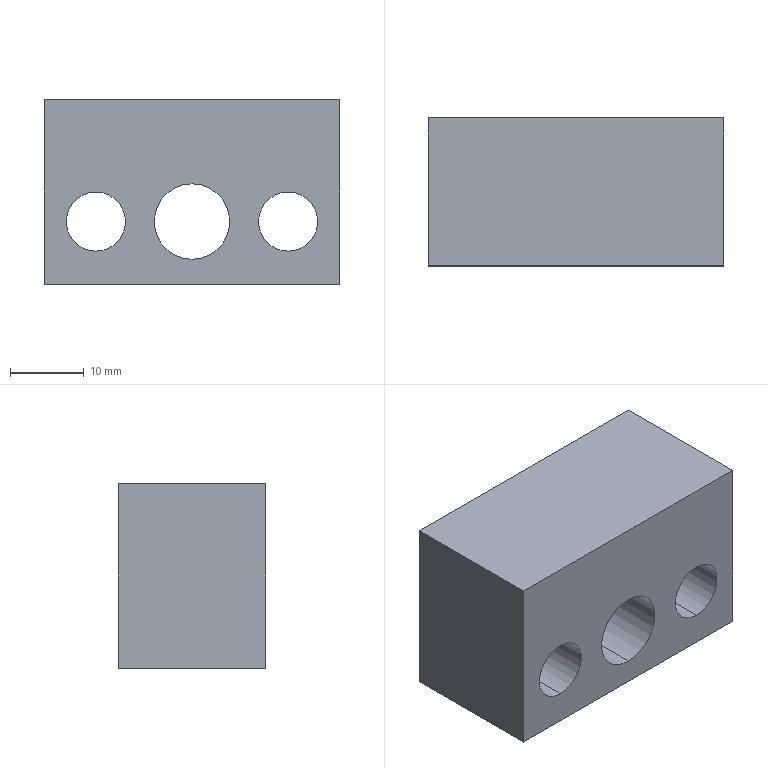Part | SolidWorks | features ICE 5, 3DProfileFeature 1, Extrusion 1, HoleWzd 1 | 1 solid | 12 faces | box 40 x 20 x 25 mm | volume 16355 mm3 | cylinder 6 | plane 6 | commonest cylinder face diameters 8 x4 10.2 x2
STEP:
#1=CARTESIAN_POINT('',(0.,-10.,-5.1));
#2=VERTEX_POINT('',#1);
#3=CARTESIAN_POINT('',(0.,-10.,5.1));
#4=VERTEX_POINT('',#3);
#5=CARTESIAN_POINT('',(0.,-10.,0.));
#6=DIRECTION('',(0.,1.,0.));
#7=DIRECTION('',(0.,0.,1.));
#8=AXIS2_PLACEMENT_3D('',#5,#6,#7);
#9=CIRCLE('',#8,5.1);
#10=EDGE_CURVE('',#2,#4,#9,.T.);
#11=ORIENTED_EDGE('',*,*,#10,.F.);
#12=CARTESIAN_POINT('',(0.,10.,-5.1));
#13=VERTEX_POINT('',#12);
#14=CARTESIAN_POINT('',(0.,10.,-5.1));
#15=DIRECTION('',(0.,1.,0.));
#16=VECTOR('',#15,1000.);
#17=LINE('',#14,#16);
#18=EDGE_CURVE('',#2,#13,#17,.T.);
#19=ORIENTED_EDGE('',*,*,#18,.T.);
#20=CARTESIAN_POINT('',(0.,10.,5.1));
#21=VERTEX_POINT('',#20);
#22=CARTESIAN_POINT('',(0.,10.,0.));
#23=DIRECTION('',(0.,1.,0.));
#24=DIRECTION('',(0.,0.,1.));
#25=AXIS2_PLACEMENT_3D('',#22,#23,#24);
#26=CIRCLE('',#25,5.1);
#27=EDGE_CURVE('',#13,#21,#26,.T.);
#28=ORIENTED_EDGE('',*,*,#27,.T.);
#29=CARTESIAN_POINT('',(0.,10.,5.1));
#30=DIRECTION('',(0.,1.,0.));
#31=VECTOR('',#30,1000.);
#32=LINE('',#29,#31);
#33=EDGE_CURVE('',#4,#21,#32,.T.);
#34=ORIENTED_EDGE('',*,*,#33,.F.);
#35=EDGE_LOOP('',(#11,#19,#28,#34));
#36=FACE_OUTER_BOUND('',#35,.T.);
#37=CARTESIAN_POINT('',(0.,10.,0.));
#38=DIRECTION('',(0.,1.,0.));
#39=DIRECTION('',(0.,0.,1.));
#40=AXIS2_PLACEMENT_3D('',#37,#38,#39);
#41=CYLINDRICAL_SURFACE('',#40,5.1);
#42=ADVANCED_FACE('',(#36),#41,.F.);
#43=CARTESIAN_POINT('',(-13.,-10.,4.));
#44=VERTEX_POINT('',#43);
#45=CARTESIAN_POINT('',(-13.,-10.,-4.));
#46=VERTEX_POINT('',#45);
#47=CARTESIAN_POINT('',(-13.,-10.,0.));
#48=DIRECTION('',(0.,-1.,0.));
#49=DIRECTION('',(0.,0.,1.));
#50=AXIS2_PLACEMENT_3D('',#47,#48,#49);
#51=CIRCLE('',#50,4.);
#52=EDGE_CURVE('',#44,#46,#51,.T.);
#53=ORIENTED_EDGE('',*,*,#52,.T.);
#54=CARTESIAN_POINT('',(-13.,10.,-4.));
#55=VERTEX_POINT('',#54);
#56=CARTESIAN_POINT('',(-13.,-10.001,-4.));
#57=DIRECTION('',(0.,1.,0.));
#58=VECTOR('',#57,1000.);
#59=LINE('',#56,#58);
#60=EDGE_CURVE('',#46,#55,#59,.T.);
#61=ORIENTED_EDGE('',*,*,#60,.T.);
#62=CARTESIAN_POINT('',(-13.,10.,4.));
#63=VERTEX_POINT('',#62);
#64=CARTESIAN_POINT('',(-13.,10.,0.));
#65=DIRECTION('',(0.,1.,0.));
#66=DIRECTION('',(0.,0.,1.));
#67=AXIS2_PLACEMENT_3D('',#64,#65,#66);
#68=CIRCLE('',#67,4.);
#69=EDGE_CURVE('',#55,#63,#68,.T.);
#70=ORIENTED_EDGE('',*,*,#69,.T.);
#71=CARTESIAN_POINT('',(-13.,-10.001,4.));
#72=DIRECTION('',(0.,1.,0.));
#73=VECTOR('',#72,1000.);
#74=LINE('',#71,#73);
#75=EDGE_CURVE('',#44,#63,#74,.T.);
#76=ORIENTED_EDGE('',*,*,#75,.F.);
#77=EDGE_LOOP('',(#53,#61,#70,#76));
#78=FACE_OUTER_BOUND('',#77,.T.);
#79=CARTESIAN_POINT('',(-13.,-10.001,0.));
#80=DIRECTION('',(0.,1.,0.));
#81=DIRECTION('',(0.,0.,1.));
#82=AXIS2_PLACEMENT_3D('',#79,#80,#81);
#83=CYLINDRICAL_SURFACE('',#82,4.);
#84=ADVANCED_FACE('',(#78),#83,.F.);
#85=CARTESIAN_POINT('',(13.,-10.,4.));
#86=VERTEX_POINT('',#85);
#87=CARTESIAN_POINT('',(13.,-10.,-4.));
#88=VERTEX_POINT('',#87);
#89=CARTESIAN_POINT('',(13.,-10.,0.));
#90=DIRECTION('',(0.,-1.,0.));
#91=DIRECTION('',(0.,0.,1.));
#92=AXIS2_PLACEMENT_3D('',#89,#90,#91);
#93=CIRCLE('',#92,4.);
#94=EDGE_CURVE('',#86,#88,#93,.T.);
#95=ORIENTED_EDGE('',*,*,#94,.T.);
#96=CARTESIAN_POINT('',(13.,10.,-4.));
#97=VERTEX_POINT('',#96);
#98=CARTESIAN_POINT('',(13.,-10.001,-4.));
#99=DIRECTION('',(0.,1.,0.));
#100=VECTOR('',#99,1000.);
#101=LINE('',#98,#100);
#102=EDGE_CURVE('',#88,#97,#101,.T.);
#103=ORIENTED_EDGE('',*,*,#102,.T.);
#104=CARTESIAN_POINT('',(13.,10.,4.));
#105=VERTEX_POINT('',#104);
#106=CARTESIAN_POINT('',(13.,10.,0.));
#107=DIRECTION('',(0.,1.,0.));
#108=DIRECTION('',(0.,0.,1.));
#109=AXIS2_PLACEMENT_3D('',#106,#107,#108);
#110=CIRCLE('',#109,4.);
#111=EDGE_CURVE('',#97,#105,#110,.T.);
#112=ORIENTED_EDGE('',*,*,#111,.T.);
#113=CARTESIAN_POINT('',(13.,-10.001,4.));
#114=DIRECTION('',(0.,1.,0.));
#115=VECTOR('',#114,1000.);
#116=LINE('',#113,#115);
#117=EDGE_CURVE('',#86,#105,#116,.T.);
#118=ORIENTED_EDGE('',*,*,#117,.F.);
#119=EDGE_LOOP('',(#95,#103,#112,#118));
#120=FACE_OUTER_BOUND('',#119,.T.);
#121=CARTESIAN_POINT('',(13.,-10.001,0.));
#122=DIRECTION('',(0.,1.,0.));
#123=DIRECTION('',(0.,0.,1.));
#124=AXIS2_PLACEMENT_3D('',#121,#122,#123);
#125=CYLINDRICAL_SURFACE('',#124,4.);
#126=ADVANCED_FACE('',(#120),#125,.F.);
#127=CARTESIAN_POINT('',(20.,-10.,-8.5));
#128=VERTEX_POINT('',#127);
#129=CARTESIAN_POINT('',(20.,10.,-8.5));
#130=VERTEX_POINT('',#129);
#131=CARTESIAN_POINT('',(20.,-10.,-8.5));
#132=DIRECTION('',(0.,1.,0.));
#133=VECTOR('',#132,1000.);
#134=LINE('',#131,#133);
#135=EDGE_CURVE('',#128,#130,#134,.T.);
#136=ORIENTED_EDGE('',*,*,#135,.T.);
#137=CARTESIAN_POINT('',(20.,10.,16.5));
#138=VERTEX_POINT('',#137);
#139=CARTESIAN_POINT('',(20.,10.,8.5));
#140=DIRECTION('',(0.,0.,-1.));
#141=VECTOR('',#140,1000.);
#142=LINE('',#139,#141);
#143=EDGE_CURVE('',#138,#130,#142,.T.);
#144=ORIENTED_EDGE('',*,*,#143,.F.);
#145=CARTESIAN_POINT('',(20.,-10.,16.5));
#146=VERTEX_POINT('',#145);
#147=CARTESIAN_POINT('',(20.,-10.,16.5));
#148=DIRECTION('',(0.,1.,0.));
#149=VECTOR('',#148,1000.);
#150=LINE('',#147,#149);
#151=EDGE_CURVE('',#146,#138,#150,.T.);
#152=ORIENTED_EDGE('',*,*,#151,.F.);
#153=CARTESIAN_POINT('',(20.,-10.,8.5));
#154=DIRECTION('',(0.,0.,-1.));
#155=VECTOR('',#154,1000.);
#156=LINE('',#153,#155);
#157=EDGE_CURVE('',#146,#128,#156,.T.);
#158=ORIENTED_EDGE('',*,*,#157,.T.);
#159=EDGE_LOOP('',(#136,#144,#152,#158));
#160=FACE_OUTER_BOUND('',#159,.T.);
#161=CARTESIAN_POINT('',(20.,-10.,8.5));
#162=DIRECTION('',(-1.,0.,0.));
#163=DIRECTION('',(0.,0.,1.));
#164=AXIS2_PLACEMENT_3D('',#161,#162,#163);
#165=PLANE('',#164);
#166=ADVANCED_FACE('',(#160),#165,.F.);
#167=CARTESIAN_POINT('',(0.,10.,0.));
#168=DIRECTION('',(0.,1.,0.));
#169=DIRECTION('',(0.,0.,1.));
#170=AXIS2_PLACEMENT_3D('',#167,#168,#169);
#171=CIRCLE('',#170,5.1);
#172=EDGE_CURVE('',#21,#13,#171,.T.);
#173=ORIENTED_EDGE('',*,*,#172,.F.);
#174=ORIENTED_EDGE('',*,*,#27,.F.);
#175=EDGE_LOOP('',(#173,#174));
#176=FACE_BOUND('',#175,.T.);
#177=CARTESIAN_POINT('',(-13.,10.,0.));
#178=DIRECTION('',(0.,1.,0.));
#179=DIRECTION('',(0.,0.,1.));
#180=AXIS2_PLACEMENT_3D('',#177,#178,#179);
#181=CIRCLE('',#180,4.);
#182=EDGE_CURVE('',#63,#55,#181,.T.);
#183=ORIENTED_EDGE('',*,*,#182,.F.);
#184=ORIENTED_EDGE('',*,*,#69,.F.);
#185=EDGE_LOOP('',(#183,#184));
#186=FACE_BOUND('',#185,.T.);
#187=CARTESIAN_POINT('',(13.,10.,0.));
#188=DIRECTION('',(0.,1.,0.));
#189=DIRECTION('',(0.,0.,1.));
#190=AXIS2_PLACEMENT_3D('',#187,#188,#189);
#191=CIRCLE('',#190,4.);
#192=EDGE_CURVE('',#105,#97,#191,.T.);
#193=ORIENTED_EDGE('',*,*,#192,.F.);
#194=ORIENTED_EDGE('',*,*,#111,.F.);
#195=EDGE_LOOP('',(#193,#194));
#196=FACE_BOUND('',#195,.T.);
#197=CARTESIAN_POINT('',(-20.,10.,-8.5));
#198=VERTEX_POINT('',#197);
#199=CARTESIAN_POINT('',(-20.,10.,-8.5));
#200=DIRECTION('',(-1.,0.,0.));
#201=VECTOR('',#200,1000.);
#202=LINE('',#199,#201);
#203=EDGE_CURVE('',#130,#198,#202,.T.);
#204=ORIENTED_EDGE('',*,*,#203,.T.);
#205=CARTESIAN_POINT('',(-20.,10.,16.5));
#206=VERTEX_POINT('',#205);
#207=CARTESIAN_POINT('',(-20.,10.,8.5));
#208=DIRECTION('',(0.,0.,-1.));
#209=VECTOR('',#208,1000.);
#210=LINE('',#207,#209);
#211=EDGE_CURVE('',#206,#198,#210,.T.);
#212=ORIENTED_EDGE('',*,*,#211,.F.);
#213=CARTESIAN_POINT('',(-20.,10.,16.5));
#214=DIRECTION('',(-1.,0.,0.));
#215=VECTOR('',#214,1000.);
#216=LINE('',#213,#215);
#217=EDGE_CURVE('',#138,#206,#216,.T.);
#218=ORIENTED_EDGE('',*,*,#217,.F.);
#219=ORIENTED_EDGE('',*,*,#143,.T.);
#220=EDGE_LOOP('',(#204,#212,#218,#219));
#221=FACE_OUTER_BOUND('',#220,.T.);
#222=CARTESIAN_POINT('',(-20.,10.,8.5));
#223=DIRECTION('',(0.,-1.,0.));
#224=DIRECTION('',(0.,0.,-1.));
#225=AXIS2_PLACEMENT_3D('',#222,#223,#224);
#226=PLANE('',#225);
#227=ADVANCED_FACE('',(#176,#186,#196,#221),#226,.F.);
#228=CARTESIAN_POINT('',(-20.,-10.,-8.5));
#229=VERTEX_POINT('',#228);
#230=CARTESIAN_POINT('',(-20.,-10.,-8.5));
#231=DIRECTION('',(0.,-1.,0.));
#232=VECTOR('',#231,1000.);
#233=LINE('',#230,#232);
#234=EDGE_CURVE('',#198,#229,#233,.T.);
#235=ORIENTED_EDGE('',*,*,#234,.T.);
#236=CARTESIAN_POINT('',(-20.,-10.,16.5));
#237=VERTEX_POINT('',#236);
#238=CARTESIAN_POINT('',(-20.,-10.,8.5));
#239=DIRECTION('',(0.,0.,-1.));
#240=VECTOR('',#239,1000.);
#241=LINE('',#238,#240);
#242=EDGE_CURVE('',#237,#229,#241,.T.);
#243=ORIENTED_EDGE('',*,*,#242,.F.);
#244=CARTESIAN_POINT('',(-20.,-10.,16.5));
#245=DIRECTION('',(0.,-1.,0.));
#246=VECTOR('',#245,1000.);
#247=LINE('',#244,#246);
#248=EDGE_CURVE('',#206,#237,#247,.T.);
#249=ORIENTED_EDGE('',*,*,#248,.F.);
#250=ORIENTED_EDGE('',*,*,#211,.T.);
#251=EDGE_LOOP('',(#235,#243,#249,#250));
#252=FACE_OUTER_BOUND('',#251,.T.);
#253=CARTESIAN_POINT('',(-20.,-10.,8.5));
#254=DIRECTION('',(1.,0.,0.));
#255=DIRECTION('',(0.,0.,-1.));
#256=AXIS2_PLACEMENT_3D('',#253,#254,#255);
#257=PLANE('',#256);
#258=ADVANCED_FACE('',(#252),#257,.F.);
#259=CARTESIAN_POINT('',(0.,-10.,0.));
#260=DIRECTION('',(0.,1.,0.));
#261=DIRECTION('',(0.,0.,1.));
#262=AXIS2_PLACEMENT_3D('',#259,#260,#261);
#263=CIRCLE('',#262,5.1);
#264=EDGE_CURVE('',#4,#2,#263,.T.);
#265=ORIENTED_EDGE('',*,*,#264,.T.);
#266=ORIENTED_EDGE('',*,*,#10,.T.);
#267=EDGE_LOOP('',(#265,#266));
#268=FACE_BOUND('',#267,.T.);
#269=ORIENTED_EDGE('',*,*,#52,.F.);
#270=CARTESIAN_POINT('',(-13.,-10.,0.));
#271=DIRECTION('',(0.,-1.,0.));
#272=DIRECTION('',(0.,0.,1.));
#273=AXIS2_PLACEMENT_3D('',#270,#271,#272);
#274=CIRCLE('',#273,4.);
#275=EDGE_CURVE('',#46,#44,#274,.T.);
#276=ORIENTED_EDGE('',*,*,#275,.F.);
#277=EDGE_LOOP('',(#269,#276));
#278=FACE_BOUND('',#277,.T.);
#279=ORIENTED_EDGE('',*,*,#94,.F.);
#280=CARTESIAN_POINT('',(13.,-10.,0.));
#281=DIRECTION('',(0.,-1.,0.));
#282=DIRECTION('',(0.,0.,1.));
#283=AXIS2_PLACEMENT_3D('',#280,#281,#282);
#284=CIRCLE('',#283,4.);
#285=EDGE_CURVE('',#88,#86,#284,.T.);
#286=ORIENTED_EDGE('',*,*,#285,.F.);
#287=EDGE_LOOP('',(#279,#286));
#288=FACE_BOUND('',#287,.T.);
#289=CARTESIAN_POINT('',(-20.,-10.,-8.5));
#290=DIRECTION('',(1.,0.,0.));
#291=VECTOR('',#290,1000.);
#292=LINE('',#289,#291);
#293=EDGE_CURVE('',#229,#128,#292,.T.);
#294=ORIENTED_EDGE('',*,*,#293,.T.);
#295=ORIENTED_EDGE('',*,*,#157,.F.);
#296=CARTESIAN_POINT('',(-20.,-10.,16.5));
#297=DIRECTION('',(1.,0.,0.));
#298=VECTOR('',#297,1000.);
#299=LINE('',#296,#298);
#300=EDGE_CURVE('',#237,#146,#299,.T.);
#301=ORIENTED_EDGE('',*,*,#300,.F.);
#302=ORIENTED_EDGE('',*,*,#242,.T.);
#303=EDGE_LOOP('',(#294,#295,#301,#302));
#304=FACE_OUTER_BOUND('',#303,.T.);
#305=CARTESIAN_POINT('',(-20.,-10.,8.5));
#306=DIRECTION('',(0.,1.,0.));
#307=DIRECTION('',(0.,0.,1.));
#308=AXIS2_PLACEMENT_3D('',#305,#306,#307);
#309=PLANE('',#308);
#310=ADVANCED_FACE('',(#268,#278,#288,#304),#309,.F.);
#311=ORIENTED_EDGE('',*,*,#135,.F.);
#312=ORIENTED_EDGE('',*,*,#293,.F.);
#313=ORIENTED_EDGE('',*,*,#234,.F.);
#314=ORIENTED_EDGE('',*,*,#203,.F.);
#315=EDGE_LOOP('',(#311,#312,#313,#314));
#316=FACE_OUTER_BOUND('',#315,.T.);
#317=CARTESIAN_POINT('',(0.,0.,-8.5));
#318=DIRECTION('',(0.,0.,-1.));
#319=DIRECTION('',(-1.,0.,0.));
#320=AXIS2_PLACEMENT_3D('',#317,#318,#319);
#321=PLANE('',#320);
#322=ADVANCED_FACE('',(#316),#321,.T.);
#323=ORIENTED_EDGE('',*,*,#102,.F.);
#324=ORIENTED_EDGE('',*,*,#285,.T.);
#325=ORIENTED_EDGE('',*,*,#117,.T.);
#326=ORIENTED_EDGE('',*,*,#192,.T.);
#327=EDGE_LOOP('',(#323,#324,#325,#326));
#328=FACE_OUTER_BOUND('',#327,.T.);
#329=CARTESIAN_POINT('',(13.,-10.001,0.));
#330=DIRECTION('',(0.,1.,0.));
#331=DIRECTION('',(0.,0.,1.));
#332=AXIS2_PLACEMENT_3D('',#329,#330,#331);
#333=CYLINDRICAL_SURFACE('',#332,4.);
#334=ADVANCED_FACE('',(#328),#333,.F.);
#335=ORIENTED_EDGE('',*,*,#60,.F.);
#336=ORIENTED_EDGE('',*,*,#275,.T.);
#337=ORIENTED_EDGE('',*,*,#75,.T.);
#338=ORIENTED_EDGE('',*,*,#182,.T.);
#339=EDGE_LOOP('',(#335,#336,#337,#338));
#340=FACE_OUTER_BOUND('',#339,.T.);
#341=CARTESIAN_POINT('',(-13.,-10.001,0.));
#342=DIRECTION('',(0.,1.,0.));
#343=DIRECTION('',(0.,0.,1.));
#344=AXIS2_PLACEMENT_3D('',#341,#342,#343);
#345=CYLINDRICAL_SURFACE('',#344,4.);
#346=ADVANCED_FACE('',(#340),#345,.F.);
#347=ORIENTED_EDGE('',*,*,#248,.T.);
#348=ORIENTED_EDGE('',*,*,#300,.T.);
#349=ORIENTED_EDGE('',*,*,#151,.T.);
#350=ORIENTED_EDGE('',*,*,#217,.T.);
#351=EDGE_LOOP('',(#347,#348,#349,#350));
#352=FACE_OUTER_BOUND('',#351,.T.);
#353=CARTESIAN_POINT('',(0.,0.,16.5));
#354=DIRECTION('',(0.,0.,-1.));
#355=DIRECTION('',(-1.,0.,0.));
#356=AXIS2_PLACEMENT_3D('',#353,#354,#355);
#357=PLANE('',#356);
#358=ADVANCED_FACE('',(#352),#357,.F.);
#359=ORIENTED_EDGE('',*,*,#18,.F.);
#360=ORIENTED_EDGE('',*,*,#264,.F.);
#361=ORIENTED_EDGE('',*,*,#33,.T.);
#362=ORIENTED_EDGE('',*,*,#172,.T.);
#363=EDGE_LOOP('',(#359,#360,#361,#362));
#364=FACE_OUTER_BOUND('',#363,.T.);
#365=CARTESIAN_POINT('',(0.,10.,0.));
#366=DIRECTION('',(0.,1.,0.));
#367=DIRECTION('',(0.,0.,1.));
#368=AXIS2_PLACEMENT_3D('',#365,#366,#367);
#369=CYLINDRICAL_SURFACE('',#368,5.1);
#370=ADVANCED_FACE('',(#364),#369,.F.);
#371=CLOSED_SHELL('',(#42,#84,#126,#166,#227,#258,#310,#322,#334,#346,#358,#370));
#372=MANIFOLD_SOLID_BREP('',#371);
#373=CARTESIAN_POINT('',(0.,0.,0.));
#374=DIRECTION('',(0.,0.,1.));
#375=DIRECTION('',(1.,0.,0.));
#376=AXIS2_PLACEMENT_3D('',#373,#374,#375);
#377=(LENGTH_UNIT()NAMED_UNIT(*)SI_UNIT(.MILLI.,.METRE.));
#378=UNCERTAINTY_MEASURE_WITH_UNIT(LENGTH_MEASURE(0.00001),#377,'','');
#379=(NAMED_UNIT(*)PLANE_ANGLE_UNIT()SI_UNIT($,.RADIAN.));
#380=(NAMED_UNIT(*)SI_UNIT($,.STERADIAN.)SOLID_ANGLE_UNIT());
#381=(GEOMETRIC_REPRESENTATION_CONTEXT(3)GLOBAL_UNCERTAINTY_ASSIGNED_CONTEXT((#378))GLOBAL_UNIT_ASSIGNED_CONTEXT((#377,#379,#380))REPRESENTATION_CONTEXT('',''));
#382=ADVANCED_BREP_SHAPE_REPRESENTATION('',(#372,#376),#381);